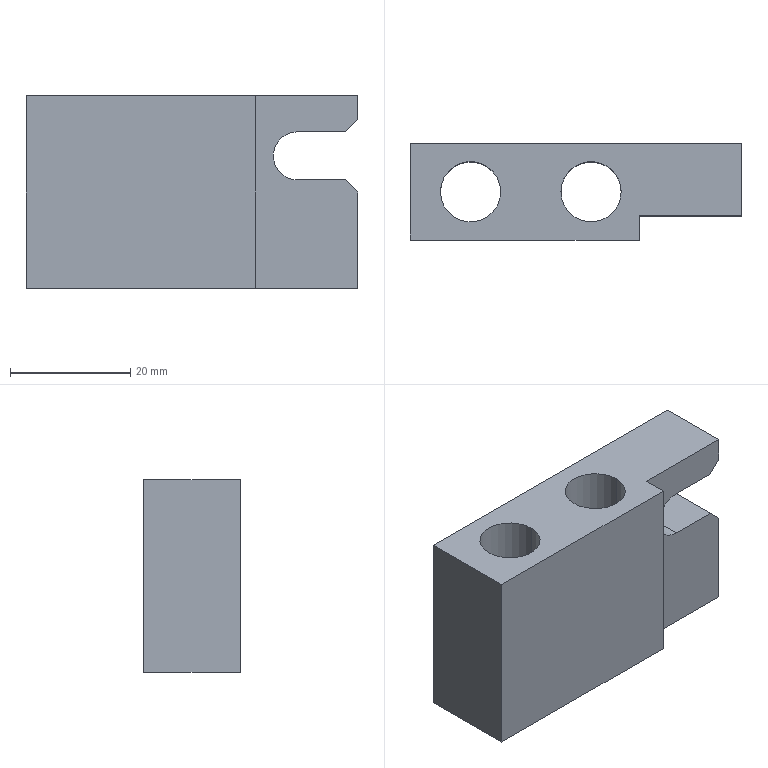Part | STEP file | J011-EBZ05-02-00-Part-1 | 1 solid | 18 faces | box 55 x 16 x 32 mm | volume 19648 mm3 | plane 13 | cylinder 5 | commonest cylinder face diameters 10 x4 8 x1
STEP:
#1=CARTESIAN_POINT('',(25.,8.,32.));
#2=VERTEX_POINT('',#1);
#3=CARTESIAN_POINT('',(35.,8.,32.));
#4=VERTEX_POINT('',#3);
#5=CARTESIAN_POINT('',(30.,8.,32.));
#6=DIRECTION('',(0.,0.,-1.));
#7=DIRECTION('',(1.,0.,0.));
#8=AXIS2_PLACEMENT_3D('',#5,#6,#7);
#9=CIRCLE('',#8,5.);
#10=EDGE_CURVE('',#2,#4,#9,.T.);
#11=ORIENTED_EDGE('',*,*,#10,.F.);
#12=CARTESIAN_POINT('',(25.,8.,0.));
#13=VERTEX_POINT('',#12);
#14=CARTESIAN_POINT('',(25.,8.,32.));
#15=DIRECTION('',(0.,0.,-1.));
#16=VECTOR('',#15,1000.);
#17=LINE('',#14,#16);
#18=EDGE_CURVE('',#2,#13,#17,.T.);
#19=ORIENTED_EDGE('',*,*,#18,.T.);
#20=CARTESIAN_POINT('',(35.,8.,0.));
#21=VERTEX_POINT('',#20);
#22=CARTESIAN_POINT('',(30.,8.,0.));
#23=DIRECTION('',(0.,0.,1.));
#24=DIRECTION('',(-1.,0.,0.));
#25=AXIS2_PLACEMENT_3D('',#22,#23,#24);
#26=CIRCLE('',#25,5.);
#27=EDGE_CURVE('',#21,#13,#26,.T.);
#28=ORIENTED_EDGE('',*,*,#27,.F.);
#29=CARTESIAN_POINT('',(35.,8.,32.));
#30=DIRECTION('',(0.,0.,-1.));
#31=VECTOR('',#30,1000.);
#32=LINE('',#29,#31);
#33=EDGE_CURVE('',#4,#21,#32,.T.);
#34=ORIENTED_EDGE('',*,*,#33,.F.);
#35=EDGE_LOOP('',(#11,#19,#28,#34));
#36=FACE_OUTER_BOUND('',#35,.T.);
#37=CARTESIAN_POINT('',(30.,8.,32.));
#38=DIRECTION('',(0.,0.,-1.));
#39=DIRECTION('',(1.,0.,0.));
#40=AXIS2_PLACEMENT_3D('',#37,#38,#39);
#41=CYLINDRICAL_SURFACE('',#40,5.);
#42=ADVANCED_FACE('',(#36),#41,.F.);
#43=CARTESIAN_POINT('',(5.,8.,32.));
#44=VERTEX_POINT('',#43);
#45=CARTESIAN_POINT('',(15.,8.,32.));
#46=VERTEX_POINT('',#45);
#47=CARTESIAN_POINT('',(10.,8.,32.));
#48=DIRECTION('',(0.,0.,-1.));
#49=DIRECTION('',(1.,0.,0.));
#50=AXIS2_PLACEMENT_3D('',#47,#48,#49);
#51=CIRCLE('',#50,5.);
#52=EDGE_CURVE('',#44,#46,#51,.T.);
#53=ORIENTED_EDGE('',*,*,#52,.F.);
#54=CARTESIAN_POINT('',(5.,8.,0.));
#55=VERTEX_POINT('',#54);
#56=CARTESIAN_POINT('',(5.,8.,32.));
#57=DIRECTION('',(0.,0.,-1.));
#58=VECTOR('',#57,1000.);
#59=LINE('',#56,#58);
#60=EDGE_CURVE('',#44,#55,#59,.T.);
#61=ORIENTED_EDGE('',*,*,#60,.T.);
#62=CARTESIAN_POINT('',(15.,8.,0.));
#63=VERTEX_POINT('',#62);
#64=CARTESIAN_POINT('',(10.,8.,0.));
#65=DIRECTION('',(0.,0.,1.));
#66=DIRECTION('',(-1.,0.,0.));
#67=AXIS2_PLACEMENT_3D('',#64,#65,#66);
#68=CIRCLE('',#67,5.);
#69=EDGE_CURVE('',#63,#55,#68,.T.);
#70=ORIENTED_EDGE('',*,*,#69,.F.);
#71=CARTESIAN_POINT('',(15.,8.,32.));
#72=DIRECTION('',(0.,0.,-1.));
#73=VECTOR('',#72,1000.);
#74=LINE('',#71,#73);
#75=EDGE_CURVE('',#46,#63,#74,.T.);
#76=ORIENTED_EDGE('',*,*,#75,.F.);
#77=EDGE_LOOP('',(#53,#61,#70,#76));
#78=FACE_OUTER_BOUND('',#77,.T.);
#79=CARTESIAN_POINT('',(10.,8.,32.));
#80=DIRECTION('',(0.,0.,-1.));
#81=DIRECTION('',(1.,0.,0.));
#82=AXIS2_PLACEMENT_3D('',#79,#80,#81);
#83=CYLINDRICAL_SURFACE('',#82,5.);
#84=ADVANCED_FACE('',(#78),#83,.F.);
#85=CARTESIAN_POINT('',(53.,16.,26.));
#86=VERTEX_POINT('',#85);
#87=CARTESIAN_POINT('',(45.,16.,26.));
#88=VERTEX_POINT('',#87);
#89=CARTESIAN_POINT('',(50.,16.,26.));
#90=DIRECTION('',(-1.,0.,0.));
#91=VECTOR('',#90,1000.);
#92=LINE('',#89,#91);
#93=EDGE_CURVE('',#86,#88,#92,.T.);
#94=ORIENTED_EDGE('',*,*,#93,.T.);
#95=CARTESIAN_POINT('',(45.,16.,18.));
#96=VERTEX_POINT('',#95);
#97=CARTESIAN_POINT('',(45.,16.,22.));
#98=DIRECTION('',(0.,-1.,0.));
#99=DIRECTION('',(0.,0.,1.));
#100=AXIS2_PLACEMENT_3D('',#97,#98,#99);
#101=CIRCLE('',#100,4.);
#102=EDGE_CURVE('',#88,#96,#101,.T.);
#103=ORIENTED_EDGE('',*,*,#102,.T.);
#104=CARTESIAN_POINT('',(53.,16.,18.));
#105=VERTEX_POINT('',#104);
#106=CARTESIAN_POINT('',(50.,16.,18.));
#107=DIRECTION('',(1.,0.,0.));
#108=VECTOR('',#107,1000.);
#109=LINE('',#106,#108);
#110=EDGE_CURVE('',#96,#105,#109,.T.);
#111=ORIENTED_EDGE('',*,*,#110,.T.);
#112=CARTESIAN_POINT('',(55.,16.,16.));
#113=VERTEX_POINT('',#112);
#114=CARTESIAN_POINT('',(49.25,16.,21.75));
#115=DIRECTION('',(0.7071,0.,-0.7071));
#116=VECTOR('',#115,1000.);
#117=LINE('',#114,#116);
#118=EDGE_CURVE('',#105,#113,#117,.T.);
#119=ORIENTED_EDGE('',*,*,#118,.T.);
#120=CARTESIAN_POINT('',(55.,16.,0.));
#121=VERTEX_POINT('',#120);
#122=CARTESIAN_POINT('',(55.,16.,0.));
#123=DIRECTION('',(0.,0.,1.));
#124=VECTOR('',#123,1000.);
#125=LINE('',#122,#124);
#126=EDGE_CURVE('',#121,#113,#125,.T.);
#127=ORIENTED_EDGE('',*,*,#126,.F.);
#128=CARTESIAN_POINT('',(0.,16.,0.));
#129=VERTEX_POINT('',#128);
#130=CARTESIAN_POINT('',(27.5,16.,0.));
#131=DIRECTION('',(-1.,0.,0.));
#132=VECTOR('',#131,1000.);
#133=LINE('',#130,#132);
#134=EDGE_CURVE('',#121,#129,#133,.T.);
#135=ORIENTED_EDGE('',*,*,#134,.T.);
#136=CARTESIAN_POINT('',(0.,16.,32.));
#137=VERTEX_POINT('',#136);
#138=CARTESIAN_POINT('',(0.,16.,0.));
#139=DIRECTION('',(0.,0.,1.));
#140=VECTOR('',#139,1000.);
#141=LINE('',#138,#140);
#142=EDGE_CURVE('',#129,#137,#141,.T.);
#143=ORIENTED_EDGE('',*,*,#142,.T.);
#144=CARTESIAN_POINT('',(55.,16.,32.));
#145=VERTEX_POINT('',#144);
#146=CARTESIAN_POINT('',(27.5,16.,32.));
#147=DIRECTION('',(1.,0.,0.));
#148=VECTOR('',#147,1000.);
#149=LINE('',#146,#148);
#150=EDGE_CURVE('',#137,#145,#149,.T.);
#151=ORIENTED_EDGE('',*,*,#150,.T.);
#152=CARTESIAN_POINT('',(55.,16.,28.));
#153=VERTEX_POINT('',#152);
#154=CARTESIAN_POINT('',(55.,16.,0.));
#155=DIRECTION('',(0.,0.,1.));
#156=VECTOR('',#155,1000.);
#157=LINE('',#154,#156);
#158=EDGE_CURVE('',#153,#145,#157,.T.);
#159=ORIENTED_EDGE('',*,*,#158,.F.);
#160=CARTESIAN_POINT('',(27.25,16.,0.25));
#161=DIRECTION('',(-0.7071,0.,-0.7071));
#162=VECTOR('',#161,1000.);
#163=LINE('',#160,#162);
#164=EDGE_CURVE('',#153,#86,#163,.T.);
#165=ORIENTED_EDGE('',*,*,#164,.T.);
#166=EDGE_LOOP('',(#94,#103,#111,#119,#127,#135,#143,#151,#159,#165));
#167=FACE_OUTER_BOUND('',#166,.T.);
#168=CARTESIAN_POINT('',(27.5,16.,0.));
#169=DIRECTION('',(0.,1.,0.));
#170=DIRECTION('',(0.,0.,-1.));
#171=AXIS2_PLACEMENT_3D('',#168,#169,#170);
#172=PLANE('',#171);
#173=ADVANCED_FACE('',(#167),#172,.T.);
#174=CARTESIAN_POINT('',(55.,4.,28.));
#175=VERTEX_POINT('',#174);
#176=CARTESIAN_POINT('',(55.,4.,32.));
#177=VERTEX_POINT('',#176);
#178=CARTESIAN_POINT('',(55.,4.,0.));
#179=DIRECTION('',(0.,0.,1.));
#180=VECTOR('',#179,1000.);
#181=LINE('',#178,#180);
#182=EDGE_CURVE('',#175,#177,#181,.T.);
#183=ORIENTED_EDGE('',*,*,#182,.F.);
#184=CARTESIAN_POINT('',(55.,16.,28.));
#185=DIRECTION('',(0.,1.,0.));
#186=VECTOR('',#185,1000.);
#187=LINE('',#184,#186);
#188=EDGE_CURVE('',#175,#153,#187,.T.);
#189=ORIENTED_EDGE('',*,*,#188,.T.);
#190=ORIENTED_EDGE('',*,*,#158,.T.);
#191=CARTESIAN_POINT('',(55.,8.,32.));
#192=DIRECTION('',(0.,-1.,0.));
#193=VECTOR('',#192,1000.);
#194=LINE('',#191,#193);
#195=EDGE_CURVE('',#145,#177,#194,.T.);
#196=ORIENTED_EDGE('',*,*,#195,.T.);
#197=EDGE_LOOP('',(#183,#189,#190,#196));
#198=FACE_OUTER_BOUND('',#197,.T.);
#199=CARTESIAN_POINT('',(55.,8.,0.));
#200=DIRECTION('',(1.,0.,0.));
#201=DIRECTION('',(0.,0.,1.));
#202=AXIS2_PLACEMENT_3D('',#199,#200,#201);
#203=PLANE('',#202);
#204=ADVANCED_FACE('',(#198),#203,.T.);
#205=CARTESIAN_POINT('',(30.,8.,32.));
#206=DIRECTION('',(0.,0.,-1.));
#207=DIRECTION('',(1.,0.,0.));
#208=AXIS2_PLACEMENT_3D('',#205,#206,#207);
#209=CIRCLE('',#208,5.);
#210=EDGE_CURVE('',#4,#2,#209,.T.);
#211=ORIENTED_EDGE('',*,*,#210,.T.);
#212=ORIENTED_EDGE('',*,*,#10,.T.);
#213=EDGE_LOOP('',(#211,#212));
#214=FACE_BOUND('',#213,.T.);
#215=CARTESIAN_POINT('',(10.,8.,32.));
#216=DIRECTION('',(0.,0.,-1.));
#217=DIRECTION('',(1.,0.,0.));
#218=AXIS2_PLACEMENT_3D('',#215,#216,#217);
#219=CIRCLE('',#218,5.);
#220=EDGE_CURVE('',#46,#44,#219,.T.);
#221=ORIENTED_EDGE('',*,*,#220,.T.);
#222=ORIENTED_EDGE('',*,*,#52,.T.);
#223=EDGE_LOOP('',(#221,#222));
#224=FACE_BOUND('',#223,.T.);
#225=CARTESIAN_POINT('',(38.,0.,32.));
#226=VERTEX_POINT('',#225);
#227=CARTESIAN_POINT('',(38.,4.,32.));
#228=VERTEX_POINT('',#227);
#229=CARTESIAN_POINT('',(38.,1.5,32.));
#230=DIRECTION('',(0.,1.,0.));
#231=VECTOR('',#230,1000.);
#232=LINE('',#229,#231);
#233=EDGE_CURVE('',#226,#228,#232,.T.);
#234=ORIENTED_EDGE('',*,*,#233,.T.);
#235=CARTESIAN_POINT('',(46.5,4.,32.));
#236=DIRECTION('',(1.,0.,0.));
#237=VECTOR('',#236,1000.);
#238=LINE('',#235,#237);
#239=EDGE_CURVE('',#228,#177,#238,.T.);
#240=ORIENTED_EDGE('',*,*,#239,.T.);
#241=ORIENTED_EDGE('',*,*,#195,.F.);
#242=ORIENTED_EDGE('',*,*,#150,.F.);
#243=CARTESIAN_POINT('',(0.,0.,32.));
#244=VERTEX_POINT('',#243);
#245=CARTESIAN_POINT('',(0.,8.,32.));
#246=DIRECTION('',(0.,1.,0.));
#247=VECTOR('',#246,1000.);
#248=LINE('',#245,#247);
#249=EDGE_CURVE('',#244,#137,#248,.T.);
#250=ORIENTED_EDGE('',*,*,#249,.F.);
#251=CARTESIAN_POINT('',(27.5,0.,32.));
#252=DIRECTION('',(-1.,0.,0.));
#253=VECTOR('',#252,1000.);
#254=LINE('',#251,#253);
#255=EDGE_CURVE('',#226,#244,#254,.T.);
#256=ORIENTED_EDGE('',*,*,#255,.F.);
#257=EDGE_LOOP('',(#234,#240,#241,#242,#250,#256));
#258=FACE_OUTER_BOUND('',#257,.T.);
#259=CARTESIAN_POINT('',(27.5,8.,32.));
#260=DIRECTION('',(0.,0.,1.));
#261=DIRECTION('',(-1.,0.,0.));
#262=AXIS2_PLACEMENT_3D('',#259,#260,#261);
#263=PLANE('',#262);
#264=ADVANCED_FACE('',(#214,#224,#258),#263,.T.);
#265=ORIENTED_EDGE('',*,*,#27,.T.);
#266=CARTESIAN_POINT('',(30.,8.,0.));
#267=DIRECTION('',(0.,0.,1.));
#268=DIRECTION('',(-1.,0.,0.));
#269=AXIS2_PLACEMENT_3D('',#266,#267,#268);
#270=CIRCLE('',#269,5.);
#271=EDGE_CURVE('',#13,#21,#270,.T.);
#272=ORIENTED_EDGE('',*,*,#271,.T.);
#273=EDGE_LOOP('',(#265,#272));
#274=FACE_BOUND('',#273,.T.);
#275=ORIENTED_EDGE('',*,*,#69,.T.);
#276=CARTESIAN_POINT('',(10.,8.,0.));
#277=DIRECTION('',(0.,0.,1.));
#278=DIRECTION('',(-1.,0.,0.));
#279=AXIS2_PLACEMENT_3D('',#276,#277,#278);
#280=CIRCLE('',#279,5.);
#281=EDGE_CURVE('',#55,#63,#280,.T.);
#282=ORIENTED_EDGE('',*,*,#281,.T.);
#283=EDGE_LOOP('',(#275,#282));
#284=FACE_BOUND('',#283,.T.);
#285=CARTESIAN_POINT('',(55.,4.,0.));
#286=VERTEX_POINT('',#285);
#287=CARTESIAN_POINT('',(38.,4.,0.));
#288=VERTEX_POINT('',#287);
#289=CARTESIAN_POINT('',(46.5,4.,0.));
#290=DIRECTION('',(-1.,0.,0.));
#291=VECTOR('',#290,1000.);
#292=LINE('',#289,#291);
#293=EDGE_CURVE('',#286,#288,#292,.T.);
#294=ORIENTED_EDGE('',*,*,#293,.T.);
#295=CARTESIAN_POINT('',(38.,0.,0.));
#296=VERTEX_POINT('',#295);
#297=CARTESIAN_POINT('',(38.,1.5,0.));
#298=DIRECTION('',(0.,-1.,0.));
#299=VECTOR('',#298,1000.);
#300=LINE('',#297,#299);
#301=EDGE_CURVE('',#288,#296,#300,.T.);
#302=ORIENTED_EDGE('',*,*,#301,.T.);
#303=CARTESIAN_POINT('',(0.,0.,0.));
#304=VERTEX_POINT('',#303);
#305=CARTESIAN_POINT('',(27.5,0.,0.));
#306=DIRECTION('',(1.,0.,0.));
#307=VECTOR('',#306,1000.);
#308=LINE('',#305,#307);
#309=EDGE_CURVE('',#304,#296,#308,.T.);
#310=ORIENTED_EDGE('',*,*,#309,.F.);
#311=CARTESIAN_POINT('',(0.,8.,0.));
#312=DIRECTION('',(0.,-1.,0.));
#313=VECTOR('',#312,1000.);
#314=LINE('',#311,#313);
#315=EDGE_CURVE('',#129,#304,#314,.T.);
#316=ORIENTED_EDGE('',*,*,#315,.F.);
#317=ORIENTED_EDGE('',*,*,#134,.F.);
#318=CARTESIAN_POINT('',(55.,8.,0.));
#319=DIRECTION('',(0.,1.,0.));
#320=VECTOR('',#319,1000.);
#321=LINE('',#318,#320);
#322=EDGE_CURVE('',#286,#121,#321,.T.);
#323=ORIENTED_EDGE('',*,*,#322,.F.);
#324=EDGE_LOOP('',(#294,#302,#310,#316,#317,#323));
#325=FACE_OUTER_BOUND('',#324,.T.);
#326=CARTESIAN_POINT('',(27.5,8.,0.));
#327=DIRECTION('',(0.,0.,-1.));
#328=DIRECTION('',(1.,0.,0.));
#329=AXIS2_PLACEMENT_3D('',#326,#327,#328);
#330=PLANE('',#329);
#331=ADVANCED_FACE('',(#274,#284,#325),#330,.T.);
#332=ORIENTED_EDGE('',*,*,#126,.T.);
#333=CARTESIAN_POINT('',(55.,4.,16.));
#334=VERTEX_POINT('',#333);
#335=CARTESIAN_POINT('',(55.,4.,16.));
#336=DIRECTION('',(0.,-1.,0.));
#337=VECTOR('',#336,1000.);
#338=LINE('',#335,#337);
#339=EDGE_CURVE('',#113,#334,#338,.T.);
#340=ORIENTED_EDGE('',*,*,#339,.T.);
#341=CARTESIAN_POINT('',(55.,4.,0.));
#342=DIRECTION('',(0.,0.,1.));
#343=VECTOR('',#342,1000.);
#344=LINE('',#341,#343);
#345=EDGE_CURVE('',#286,#334,#344,.T.);
#346=ORIENTED_EDGE('',*,*,#345,.F.);
#347=ORIENTED_EDGE('',*,*,#322,.T.);
#348=EDGE_LOOP('',(#332,#340,#346,#347));
#349=FACE_OUTER_BOUND('',#348,.T.);
#350=CARTESIAN_POINT('',(55.,8.,0.));
#351=DIRECTION('',(1.,0.,0.));
#352=DIRECTION('',(0.,0.,1.));
#353=AXIS2_PLACEMENT_3D('',#350,#351,#352);
#354=PLANE('',#353);
#355=ADVANCED_FACE('',(#349),#354,.T.);
#356=CARTESIAN_POINT('',(38.,0.,0.));
#357=DIRECTION('',(0.,0.,-1.));
#358=VECTOR('',#357,1000.);
#359=LINE('',#356,#358);
#360=EDGE_CURVE('',#226,#296,#359,.T.);
#361=ORIENTED_EDGE('',*,*,#360,.F.);
#362=ORIENTED_EDGE('',*,*,#255,.T.);
#363=CARTESIAN_POINT('',(0.,0.,0.));
#364=DIRECTION('',(0.,0.,1.));
#365=VECTOR('',#364,1000.);
#366=LINE('',#363,#365);
#367=EDGE_CURVE('',#304,#244,#366,.T.);
#368=ORIENTED_EDGE('',*,*,#367,.F.);
#369=ORIENTED_EDGE('',*,*,#309,.T.);
#370=EDGE_LOOP('',(#361,#362,#368,#369));
#371=FACE_OUTER_BOUND('',#370,.T.);
#372=CARTESIAN_POINT('',(27.5,0.,0.));
#373=DIRECTION('',(0.,-1.,0.));
#374=DIRECTION('',(0.,0.,1.));
#375=AXIS2_PLACEMENT_3D('',#372,#373,#374);
#376=PLANE('',#375);
#377=ADVANCED_FACE('',(#371),#376,.T.);
#378=ORIENTED_EDGE('',*,*,#315,.T.);
#379=ORIENTED_EDGE('',*,*,#367,.T.);
#380=ORIENTED_EDGE('',*,*,#249,.T.);
#381=ORIENTED_EDGE('',*,*,#142,.F.);
#382=EDGE_LOOP('',(#378,#379,#380,#381));
#383=FACE_OUTER_BOUND('',#382,.T.);
#384=CARTESIAN_POINT('',(0.,8.,0.));
#385=DIRECTION('',(-1.,0.,0.));
#386=DIRECTION('',(0.,0.,-1.));
#387=AXIS2_PLACEMENT_3D('',#384,#385,#386);
#388=PLANE('',#387);
#389=ADVANCED_FACE('',(#383),#388,.T.);
#390=CARTESIAN_POINT('',(53.,4.,18.));
#391=VERTEX_POINT('',#390);
#392=CARTESIAN_POINT('',(45.,4.,18.));
#393=VERTEX_POINT('',#392);
#394=CARTESIAN_POINT('',(46.5,4.,18.));
#395=DIRECTION('',(-1.,0.,0.));
#396=VECTOR('',#395,1000.);
#397=LINE('',#394,#396);
#398=EDGE_CURVE('',#391,#393,#397,.T.);
#399=ORIENTED_EDGE('',*,*,#398,.T.);
#400=CARTESIAN_POINT('',(45.,4.,26.));
#401=VERTEX_POINT('',#400);
#402=CARTESIAN_POINT('',(45.,4.,22.));
#403=DIRECTION('',(0.,1.,0.));
#404=DIRECTION('',(0.,0.,-1.));
#405=AXIS2_PLACEMENT_3D('',#402,#403,#404);
#406=CIRCLE('',#405,4.);
#407=EDGE_CURVE('',#393,#401,#406,.T.);
#408=ORIENTED_EDGE('',*,*,#407,.T.);
#409=CARTESIAN_POINT('',(53.,4.,26.));
#410=VERTEX_POINT('',#409);
#411=CARTESIAN_POINT('',(46.5,4.,26.));
#412=DIRECTION('',(1.,0.,0.));
#413=VECTOR('',#412,1000.);
#414=LINE('',#411,#413);
#415=EDGE_CURVE('',#401,#410,#414,.T.);
#416=ORIENTED_EDGE('',*,*,#415,.T.);
#417=CARTESIAN_POINT('',(55.,4.,28.));
#418=DIRECTION('',(0.7071,0.,0.7071));
#419=VECTOR('',#418,1000.);
#420=LINE('',#417,#419);
#421=EDGE_CURVE('',#410,#175,#420,.T.);
#422=ORIENTED_EDGE('',*,*,#421,.T.);
#423=ORIENTED_EDGE('',*,*,#182,.T.);
#424=ORIENTED_EDGE('',*,*,#239,.F.);
#425=CARTESIAN_POINT('',(38.,4.,0.));
#426=DIRECTION('',(0.,0.,1.));
#427=VECTOR('',#426,1000.);
#428=LINE('',#425,#427);
#429=EDGE_CURVE('',#288,#228,#428,.T.);
#430=ORIENTED_EDGE('',*,*,#429,.F.);
#431=ORIENTED_EDGE('',*,*,#293,.F.);
#432=ORIENTED_EDGE('',*,*,#345,.T.);
#433=CARTESIAN_POINT('',(53.,4.,18.));
#434=DIRECTION('',(-0.7071,0.,0.7071));
#435=VECTOR('',#434,1000.);
#436=LINE('',#433,#435);
#437=EDGE_CURVE('',#334,#391,#436,.T.);
#438=ORIENTED_EDGE('',*,*,#437,.T.);
#439=EDGE_LOOP('',(#399,#408,#416,#422,#423,#424,#430,#431,#432,#438));
#440=FACE_OUTER_BOUND('',#439,.T.);
#441=CARTESIAN_POINT('',(46.5,4.,0.));
#442=DIRECTION('',(0.,1.,0.));
#443=DIRECTION('',(0.,0.,-1.));
#444=AXIS2_PLACEMENT_3D('',#441,#442,#443);
#445=PLANE('',#444);
#446=ADVANCED_FACE('',(#440),#445,.F.);
#447=ORIENTED_EDGE('',*,*,#360,.T.);
#448=ORIENTED_EDGE('',*,*,#301,.F.);
#449=ORIENTED_EDGE('',*,*,#429,.T.);
#450=ORIENTED_EDGE('',*,*,#233,.F.);
#451=EDGE_LOOP('',(#447,#448,#449,#450));
#452=FACE_OUTER_BOUND('',#451,.T.);
#453=CARTESIAN_POINT('',(38.,1.5,0.));
#454=DIRECTION('',(-1.,0.,0.));
#455=DIRECTION('',(0.,0.,-1.));
#456=AXIS2_PLACEMENT_3D('',#453,#454,#455);
#457=PLANE('',#456);
#458=ADVANCED_FACE('',(#452),#457,.F.);
#459=ORIENTED_EDGE('',*,*,#60,.F.);
#460=ORIENTED_EDGE('',*,*,#220,.F.);
#461=ORIENTED_EDGE('',*,*,#75,.T.);
#462=ORIENTED_EDGE('',*,*,#281,.F.);
#463=EDGE_LOOP('',(#459,#460,#461,#462));
#464=FACE_OUTER_BOUND('',#463,.T.);
#465=CARTESIAN_POINT('',(10.,8.,32.));
#466=DIRECTION('',(0.,0.,-1.));
#467=DIRECTION('',(1.,0.,0.));
#468=AXIS2_PLACEMENT_3D('',#465,#466,#467);
#469=CYLINDRICAL_SURFACE('',#468,5.);
#470=ADVANCED_FACE('',(#464),#469,.F.);
#471=ORIENTED_EDGE('',*,*,#18,.F.);
#472=ORIENTED_EDGE('',*,*,#210,.F.);
#473=ORIENTED_EDGE('',*,*,#33,.T.);
#474=ORIENTED_EDGE('',*,*,#271,.F.);
#475=EDGE_LOOP('',(#471,#472,#473,#474));
#476=FACE_OUTER_BOUND('',#475,.T.);
#477=CARTESIAN_POINT('',(30.,8.,32.));
#478=DIRECTION('',(0.,0.,-1.));
#479=DIRECTION('',(1.,0.,0.));
#480=AXIS2_PLACEMENT_3D('',#477,#478,#479);
#481=CYLINDRICAL_SURFACE('',#480,5.);
#482=ADVANCED_FACE('',(#476),#481,.F.);
#483=ORIENTED_EDGE('',*,*,#398,.F.);
#484=CARTESIAN_POINT('',(53.,16.,18.));
#485=DIRECTION('',(0.,1.,0.));
#486=VECTOR('',#485,1000.);
#487=LINE('',#484,#486);
#488=EDGE_CURVE('',#391,#105,#487,.T.);
#489=ORIENTED_EDGE('',*,*,#488,.T.);
#490=ORIENTED_EDGE('',*,*,#110,.F.);
#491=CARTESIAN_POINT('',(45.,0.,18.));
#492=DIRECTION('',(0.,1.,0.));
#493=VECTOR('',#492,1000.);
#494=LINE('',#491,#493);
#495=EDGE_CURVE('',#393,#96,#494,.T.);
#496=ORIENTED_EDGE('',*,*,#495,.F.);
#497=EDGE_LOOP('',(#483,#489,#490,#496));
#498=FACE_OUTER_BOUND('',#497,.T.);
#499=CARTESIAN_POINT('',(50.,0.,18.));
#500=DIRECTION('',(0.,0.,-1.));
#501=DIRECTION('',(0.,-1.,0.));
#502=AXIS2_PLACEMENT_3D('',#499,#500,#501);
#503=PLANE('',#502);
#504=ADVANCED_FACE('',(#498),#503,.F.);
#505=ORIENTED_EDGE('',*,*,#93,.F.);
#506=CARTESIAN_POINT('',(53.,4.,26.));
#507=DIRECTION('',(0.,-1.,0.));
#508=VECTOR('',#507,1000.);
#509=LINE('',#506,#508);
#510=EDGE_CURVE('',#86,#410,#509,.T.);
#511=ORIENTED_EDGE('',*,*,#510,.T.);
#512=ORIENTED_EDGE('',*,*,#415,.F.);
#513=CARTESIAN_POINT('',(45.,0.,26.));
#514=DIRECTION('',(0.,1.,0.));
#515=VECTOR('',#514,1000.);
#516=LINE('',#513,#515);
#517=EDGE_CURVE('',#401,#88,#516,.T.);
#518=ORIENTED_EDGE('',*,*,#517,.T.);
#519=EDGE_LOOP('',(#505,#511,#512,#518));
#520=FACE_OUTER_BOUND('',#519,.T.);
#521=CARTESIAN_POINT('',(50.,0.,26.));
#522=DIRECTION('',(0.,0.,1.));
#523=DIRECTION('',(0.,1.,0.));
#524=AXIS2_PLACEMENT_3D('',#521,#522,#523);
#525=PLANE('',#524);
#526=ADVANCED_FACE('',(#520),#525,.F.);
#527=ORIENTED_EDGE('',*,*,#421,.F.);
#528=ORIENTED_EDGE('',*,*,#510,.F.);
#529=ORIENTED_EDGE('',*,*,#164,.F.);
#530=ORIENTED_EDGE('',*,*,#188,.F.);
#531=EDGE_LOOP('',(#527,#528,#529,#530));
#532=FACE_OUTER_BOUND('',#531,.T.);
#533=CARTESIAN_POINT('',(55.,8.,28.));
#534=DIRECTION('',(0.7071,0.,-0.7071));
#535=DIRECTION('',(0.,-1.,0.));
#536=AXIS2_PLACEMENT_3D('',#533,#534,#535);
#537=PLANE('',#536);
#538=ADVANCED_FACE('',(#532),#537,.T.);
#539=ORIENTED_EDGE('',*,*,#437,.F.);
#540=ORIENTED_EDGE('',*,*,#339,.F.);
#541=ORIENTED_EDGE('',*,*,#118,.F.);
#542=ORIENTED_EDGE('',*,*,#488,.F.);
#543=EDGE_LOOP('',(#539,#540,#541,#542));
#544=FACE_OUTER_BOUND('',#543,.T.);
#545=CARTESIAN_POINT('',(53.,0.,18.));
#546=DIRECTION('',(0.7071,0.,0.7071));
#547=DIRECTION('',(0.,-1.,0.));
#548=AXIS2_PLACEMENT_3D('',#545,#546,#547);
#549=PLANE('',#548);
#550=ADVANCED_FACE('',(#544),#549,.T.);
#551=ORIENTED_EDGE('',*,*,#102,.F.);
#552=ORIENTED_EDGE('',*,*,#517,.F.);
#553=ORIENTED_EDGE('',*,*,#407,.F.);
#554=ORIENTED_EDGE('',*,*,#495,.T.);
#555=EDGE_LOOP('',(#551,#552,#553,#554));
#556=FACE_OUTER_BOUND('',#555,.T.);
#557=CARTESIAN_POINT('',(45.,16.,22.));
#558=DIRECTION('',(0.,-1.,0.));
#559=DIRECTION('',(0.,0.,1.));
#560=AXIS2_PLACEMENT_3D('',#557,#558,#559);
#561=CYLINDRICAL_SURFACE('',#560,4.);
#562=ADVANCED_FACE('',(#556),#561,.F.);
#563=CLOSED_SHELL('',(#42,#84,#173,#204,#264,#331,#355,#377,#389,#446,#458,#470,#482,#504,#526,#538,#550,#562));
#564=MANIFOLD_SOLID_BREP('',#563);
#565=CARTESIAN_POINT('',(0.,0.,0.));
#566=DIRECTION('',(0.,0.,1.));
#567=DIRECTION('',(1.,0.,0.));
#568=AXIS2_PLACEMENT_3D('',#565,#566,#567);
#569=(LENGTH_UNIT()NAMED_UNIT(*)SI_UNIT(.MILLI.,.METRE.));
#570=UNCERTAINTY_MEASURE_WITH_UNIT(LENGTH_MEASURE(0.00001),#569,'','');
#571=(NAMED_UNIT(*)PLANE_ANGLE_UNIT()SI_UNIT($,.RADIAN.));
#572=(NAMED_UNIT(*)SI_UNIT($,.STERADIAN.)SOLID_ANGLE_UNIT());
#573=(GEOMETRIC_REPRESENTATION_CONTEXT(3)GLOBAL_UNCERTAINTY_ASSIGNED_CONTEXT((#570))GLOBAL_UNIT_ASSIGNED_CONTEXT((#569,#571,#572))REPRESENTATION_CONTEXT('',''));
#574=ADVANCED_BREP_SHAPE_REPRESENTATION('',(#564,#568),#573);